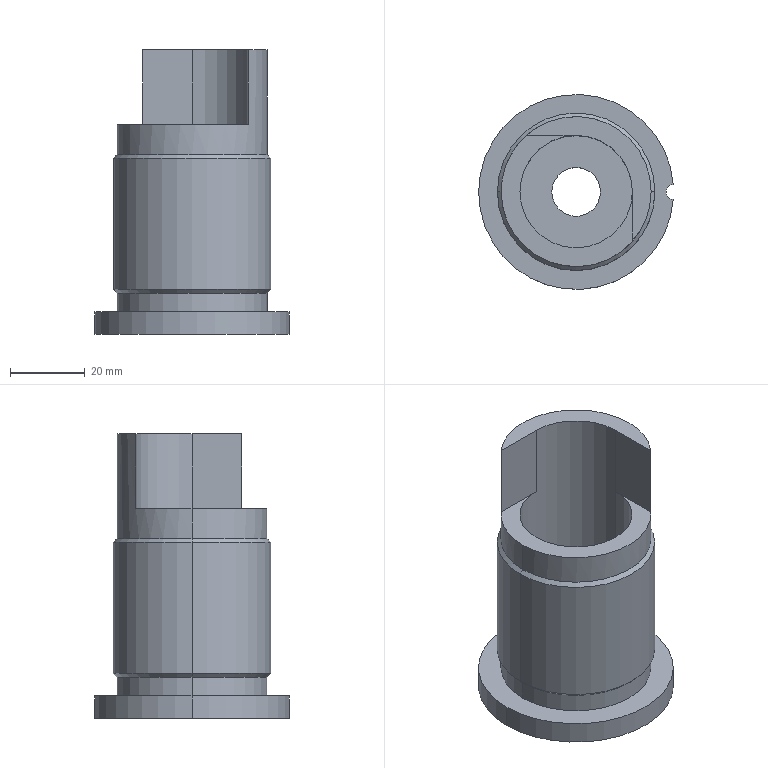Part | SolidWorks | features ICE 8, Chamfer 3, Extrusion 1 | 1 solid | 30 faces | box 51.923 x 52 x 76 mm | volume 55221 mm3 | cylinder 15 | cone 8 | plane 7 | commonest cylinder face diameters 40 x4 13 x2 30 x2 32 x2 42 x2 52 x2
STEP:
#1=CARTESIAN_POINT('',(15.,0.,21.));
#2=VERTEX_POINT('',#1);
#3=CARTESIAN_POINT('',(-15.,0.,21.));
#4=VERTEX_POINT('',#3);
#5=CARTESIAN_POINT('',(0.,0.,21.));
#6=DIRECTION('',(0.,0.,-1.));
#7=DIRECTION('',(1.,0.,0.));
#8=AXIS2_PLACEMENT_3D('',#5,#6,#7);
#9=CIRCLE('',#8,15.);
#10=EDGE_CURVE('',#2,#4,#9,.T.);
#11=ORIENTED_EDGE('',*,*,#10,.F.);
#12=CARTESIAN_POINT('',(16.,0.,20.));
#13=VERTEX_POINT('',#12);
#14=CARTESIAN_POINT('',(16.,0.,20.));
#15=DIRECTION('',(0.7071,0.,-0.7071));
#16=VECTOR('',#15,1000.);
#17=LINE('',#14,#16);
#18=EDGE_CURVE('',#2,#13,#17,.T.);
#19=ORIENTED_EDGE('',*,*,#18,.T.);
#20=CARTESIAN_POINT('',(-16.,0.,20.));
#21=VERTEX_POINT('',#20);
#22=CARTESIAN_POINT('',(0.,0.,20.));
#23=DIRECTION('',(0.,0.,1.));
#24=DIRECTION('',(1.,0.,0.));
#25=AXIS2_PLACEMENT_3D('',#22,#23,#24);
#26=CIRCLE('',#25,16.);
#27=EDGE_CURVE('',#21,#13,#26,.T.);
#28=ORIENTED_EDGE('',*,*,#27,.F.);
#29=CARTESIAN_POINT('',(-16.,0.,20.));
#30=DIRECTION('',(-0.7071,0.,-0.7071));
#31=VECTOR('',#30,1000.);
#32=LINE('',#29,#31);
#33=EDGE_CURVE('',#4,#21,#32,.T.);
#34=ORIENTED_EDGE('',*,*,#33,.F.);
#35=EDGE_LOOP('',(#11,#19,#28,#34));
#36=FACE_OUTER_BOUND('',#35,.T.);
#37=CARTESIAN_POINT('',(0.,0.,20.));
#38=DIRECTION('',(0.,0.,-1.));
#39=DIRECTION('',(-1.,0.,0.));
#40=AXIS2_PLACEMENT_3D('',#37,#38,#39);
#41=CONICAL_SURFACE('',#40,16.,0.7854);
#42=ADVANCED_FACE('',(#36),#41,.F.);
#43=CARTESIAN_POINT('',(6.5,0.,1.));
#44=VERTEX_POINT('',#43);
#45=CARTESIAN_POINT('',(-6.5,0.,1.));
#46=VERTEX_POINT('',#45);
#47=CARTESIAN_POINT('',(0.,0.,1.));
#48=DIRECTION('',(0.,0.,-1.));
#49=DIRECTION('',(1.,0.,0.));
#50=AXIS2_PLACEMENT_3D('',#47,#48,#49);
#51=CIRCLE('',#50,6.5);
#52=EDGE_CURVE('',#44,#46,#51,.T.);
#53=ORIENTED_EDGE('',*,*,#52,.F.);
#54=CARTESIAN_POINT('',(7.5,0.,0.));
#55=VERTEX_POINT('',#54);
#56=CARTESIAN_POINT('',(7.5,0.,0.));
#57=DIRECTION('',(0.7071,0.,-0.7071));
#58=VECTOR('',#57,1000.);
#59=LINE('',#56,#58);
#60=EDGE_CURVE('',#44,#55,#59,.T.);
#61=ORIENTED_EDGE('',*,*,#60,.T.);
#62=CARTESIAN_POINT('',(-7.5,0.,0.));
#63=VERTEX_POINT('',#62);
#64=CARTESIAN_POINT('',(0.,0.,0.));
#65=DIRECTION('',(0.,0.,1.));
#66=DIRECTION('',(1.,0.,0.));
#67=AXIS2_PLACEMENT_3D('',#64,#65,#66);
#68=CIRCLE('',#67,7.5);
#69=EDGE_CURVE('',#63,#55,#68,.T.);
#70=ORIENTED_EDGE('',*,*,#69,.F.);
#71=CARTESIAN_POINT('',(-7.5,0.,0.));
#72=DIRECTION('',(-0.7071,0.,-0.7071));
#73=VECTOR('',#72,1000.);
#74=LINE('',#71,#73);
#75=EDGE_CURVE('',#46,#63,#74,.T.);
#76=ORIENTED_EDGE('',*,*,#75,.F.);
#77=EDGE_LOOP('',(#53,#61,#70,#76));
#78=FACE_OUTER_BOUND('',#77,.T.);
#79=CARTESIAN_POINT('',(0.,0.,0.));
#80=DIRECTION('',(0.,0.,-1.));
#81=DIRECTION('',(-1.,0.,0.));
#82=AXIS2_PLACEMENT_3D('',#79,#80,#81);
#83=CONICAL_SURFACE('',#82,7.5,0.7854);
#84=ADVANCED_FACE('',(#78),#83,.F.);
#85=ORIENTED_EDGE('',*,*,#52,.T.);
#86=CARTESIAN_POINT('',(-6.5,0.,18.));
#87=VERTEX_POINT('',#86);
#88=CARTESIAN_POINT('',(-6.5,0.,-5.));
#89=DIRECTION('',(0.,0.,1.));
#90=VECTOR('',#89,1000.);
#91=LINE('',#88,#90);
#92=EDGE_CURVE('',#46,#87,#91,.T.);
#93=ORIENTED_EDGE('',*,*,#92,.T.);
#94=CARTESIAN_POINT('',(6.5,0.,18.));
#95=VERTEX_POINT('',#94);
#96=CARTESIAN_POINT('',(0.,0.,18.));
#97=DIRECTION('',(0.,0.,1.));
#98=DIRECTION('',(1.,0.,0.));
#99=AXIS2_PLACEMENT_3D('',#96,#97,#98);
#100=CIRCLE('',#99,6.5);
#101=EDGE_CURVE('',#87,#95,#100,.T.);
#102=ORIENTED_EDGE('',*,*,#101,.T.);
#103=CARTESIAN_POINT('',(6.5,0.,-5.));
#104=DIRECTION('',(0.,0.,1.));
#105=VECTOR('',#104,1000.);
#106=LINE('',#103,#105);
#107=EDGE_CURVE('',#44,#95,#106,.T.);
#108=ORIENTED_EDGE('',*,*,#107,.F.);
#109=EDGE_LOOP('',(#85,#93,#102,#108));
#110=FACE_OUTER_BOUND('',#109,.T.);
#111=CARTESIAN_POINT('',(0.,0.,-5.));
#112=DIRECTION('',(0.,0.,1.));
#113=DIRECTION('',(1.,0.,0.));
#114=AXIS2_PLACEMENT_3D('',#111,#112,#113);
#115=CYLINDRICAL_SURFACE('',#114,6.5);
#116=ADVANCED_FACE('',(#110),#115,.F.);
#117=ORIENTED_EDGE('',*,*,#27,.T.);
#118=CARTESIAN_POINT('',(16.,0.,18.));
#119=VERTEX_POINT('',#118);
#120=CARTESIAN_POINT('',(16.,0.,21.));
#121=DIRECTION('',(0.,0.,-1.));
#122=VECTOR('',#121,1000.);
#123=LINE('',#120,#122);
#124=EDGE_CURVE('',#13,#119,#123,.T.);
#125=ORIENTED_EDGE('',*,*,#124,.T.);
#126=CARTESIAN_POINT('',(-16.,0.,18.));
#127=VERTEX_POINT('',#126);
#128=CARTESIAN_POINT('',(0.,0.,18.));
#129=DIRECTION('',(0.,0.,1.));
#130=DIRECTION('',(1.,0.,0.));
#131=AXIS2_PLACEMENT_3D('',#128,#129,#130);
#132=CIRCLE('',#131,16.);
#133=EDGE_CURVE('',#127,#119,#132,.T.);
#134=ORIENTED_EDGE('',*,*,#133,.F.);
#135=CARTESIAN_POINT('',(-16.,0.,21.));
#136=DIRECTION('',(0.,0.,-1.));
#137=VECTOR('',#136,1000.);
#138=LINE('',#135,#137);
#139=EDGE_CURVE('',#21,#127,#138,.T.);
#140=ORIENTED_EDGE('',*,*,#139,.F.);
#141=EDGE_LOOP('',(#117,#125,#134,#140));
#142=FACE_OUTER_BOUND('',#141,.T.);
#143=CARTESIAN_POINT('',(0.,0.,21.));
#144=DIRECTION('',(0.,0.,-1.));
#145=DIRECTION('',(-1.,0.,0.));
#146=AXIS2_PLACEMENT_3D('',#143,#144,#145);
#147=CYLINDRICAL_SURFACE('',#146,16.);
#148=ADVANCED_FACE('',(#142),#147,.F.);
#149=CARTESIAN_POINT('',(-20.,0.,48.));
#150=VERTEX_POINT('',#149);
#151=CARTESIAN_POINT('',(20.,0.,48.));
#152=VERTEX_POINT('',#151);
#153=CARTESIAN_POINT('',(0.,0.,48.));
#154=DIRECTION('',(0.,0.,-1.));
#155=DIRECTION('',(1.,0.,0.));
#156=AXIS2_PLACEMENT_3D('',#153,#154,#155);
#157=CIRCLE('',#156,20.);
#158=EDGE_CURVE('',#150,#152,#157,.T.);
#159=ORIENTED_EDGE('',*,*,#158,.T.);
#160=CARTESIAN_POINT('',(21.,0.,47.));
#161=VERTEX_POINT('',#160);
#162=CARTESIAN_POINT('',(20.,0.,48.));
#163=DIRECTION('',(0.7071,0.,-0.7071));
#164=VECTOR('',#163,1000.);
#165=LINE('',#162,#164);
#166=EDGE_CURVE('',#152,#161,#165,.T.);
#167=ORIENTED_EDGE('',*,*,#166,.T.);
#168=CARTESIAN_POINT('',(-21.,0.,47.));
#169=VERTEX_POINT('',#168);
#170=CARTESIAN_POINT('',(0.,0.,47.));
#171=DIRECTION('',(0.,0.,-1.));
#172=DIRECTION('',(1.,0.,0.));
#173=AXIS2_PLACEMENT_3D('',#170,#171,#172);
#174=CIRCLE('',#173,21.);
#175=EDGE_CURVE('',#169,#161,#174,.T.);
#176=ORIENTED_EDGE('',*,*,#175,.F.);
#177=CARTESIAN_POINT('',(-20.,0.,48.));
#178=DIRECTION('',(-0.7071,0.,-0.7071));
#179=VECTOR('',#178,1000.);
#180=LINE('',#177,#179);
#181=EDGE_CURVE('',#150,#169,#180,.T.);
#182=ORIENTED_EDGE('',*,*,#181,.F.);
#183=EDGE_LOOP('',(#159,#167,#176,#182));
#184=FACE_OUTER_BOUND('',#183,.T.);
#185=CARTESIAN_POINT('',(0.,0.,48.));
#186=DIRECTION('',(0.,0.,-1.));
#187=DIRECTION('',(-1.,0.,0.));
#188=AXIS2_PLACEMENT_3D('',#185,#186,#187);
#189=CONICAL_SURFACE('',#188,20.,0.7854);
#190=ADVANCED_FACE('',(#184),#189,.T.);
#191=CARTESIAN_POINT('',(20.,0.,11.));
#192=VERTEX_POINT('',#191);
#193=CARTESIAN_POINT('',(-20.,0.,11.));
#194=VERTEX_POINT('',#193);
#195=CARTESIAN_POINT('',(0.,0.,11.));
#196=DIRECTION('',(0.,0.,1.));
#197=DIRECTION('',(1.,0.,0.));
#198=AXIS2_PLACEMENT_3D('',#195,#196,#197);
#199=CIRCLE('',#198,20.);
#200=EDGE_CURVE('',#192,#194,#199,.T.);
#201=ORIENTED_EDGE('',*,*,#200,.T.);
#202=CARTESIAN_POINT('',(-21.,0.,12.));
#203=VERTEX_POINT('',#202);
#204=CARTESIAN_POINT('',(-21.,0.,12.));
#205=DIRECTION('',(-0.7071,0.,0.7071));
#206=VECTOR('',#205,1000.);
#207=LINE('',#204,#206);
#208=EDGE_CURVE('',#194,#203,#207,.T.);
#209=ORIENTED_EDGE('',*,*,#208,.T.);
#210=CARTESIAN_POINT('',(21.,0.,12.));
#211=VERTEX_POINT('',#210);
#212=CARTESIAN_POINT('',(0.,0.,12.));
#213=DIRECTION('',(0.,0.,1.));
#214=DIRECTION('',(1.,0.,0.));
#215=AXIS2_PLACEMENT_3D('',#212,#213,#214);
#216=CIRCLE('',#215,21.);
#217=EDGE_CURVE('',#211,#203,#216,.T.);
#218=ORIENTED_EDGE('',*,*,#217,.F.);
#219=CARTESIAN_POINT('',(21.,0.,12.));
#220=DIRECTION('',(0.7071,0.,0.7071));
#221=VECTOR('',#220,1000.);
#222=LINE('',#219,#221);
#223=EDGE_CURVE('',#192,#211,#222,.T.);
#224=ORIENTED_EDGE('',*,*,#223,.F.);
#225=EDGE_LOOP('',(#201,#209,#218,#224));
#226=FACE_OUTER_BOUND('',#225,.T.);
#227=CARTESIAN_POINT('',(0.,0.,12.));
#228=DIRECTION('',(0.,0.,1.));
#229=DIRECTION('',(1.,0.,0.));
#230=AXIS2_PLACEMENT_3D('',#227,#228,#229);
#231=CONICAL_SURFACE('',#230,21.,0.7854);
#232=ADVANCED_FACE('',(#226),#231,.T.);
#233=CARTESIAN_POINT('',(20.,0.,76.));
#234=VERTEX_POINT('',#233);
#235=CARTESIAN_POINT('',(-13.229,15.,76.));
#236=VERTEX_POINT('',#235);
#237=CARTESIAN_POINT('',(0.,0.,76.));
#238=DIRECTION('',(0.,0.,1.));
#239=DIRECTION('',(1.,0.,0.));
#240=AXIS2_PLACEMENT_3D('',#237,#238,#239);
#241=CIRCLE('',#240,20.);
#242=EDGE_CURVE('',#234,#236,#241,.T.);
#243=ORIENTED_EDGE('',*,*,#242,.F.);
#244=CARTESIAN_POINT('',(20.,0.,76.));
#245=DIRECTION('',(0.,0.,-1.));
#246=VECTOR('',#245,1000.);
#247=LINE('',#244,#246);
#248=EDGE_CURVE('',#234,#152,#247,.T.);
#249=ORIENTED_EDGE('',*,*,#248,.T.);
#250=ORIENTED_EDGE('',*,*,#158,.F.);
#251=CARTESIAN_POINT('',(-20.,0.,56.));
#252=VERTEX_POINT('',#251);
#253=CARTESIAN_POINT('',(-20.,0.,76.));
#254=DIRECTION('',(0.,0.,-1.));
#255=VECTOR('',#254,1000.);
#256=LINE('',#253,#255);
#257=EDGE_CURVE('',#252,#150,#256,.T.);
#258=ORIENTED_EDGE('',*,*,#257,.F.);
#259=CARTESIAN_POINT('',(-13.229,15.,56.));
#260=VERTEX_POINT('',#259);
#261=CARTESIAN_POINT('',(0.,0.,56.));
#262=DIRECTION('',(0.,0.,1.));
#263=DIRECTION('',(1.,0.,0.));
#264=AXIS2_PLACEMENT_3D('',#261,#262,#263);
#265=CIRCLE('',#264,20.);
#266=EDGE_CURVE('',#260,#252,#265,.T.);
#267=ORIENTED_EDGE('',*,*,#266,.F.);
#268=CARTESIAN_POINT('',(-13.229,15.,76.));
#269=DIRECTION('',(0.,0.,1.));
#270=VECTOR('',#269,1000.);
#271=LINE('',#268,#270);
#272=EDGE_CURVE('',#260,#236,#271,.T.);
#273=ORIENTED_EDGE('',*,*,#272,.T.);
#274=EDGE_LOOP('',(#243,#249,#250,#258,#267,#273));
#275=FACE_OUTER_BOUND('',#274,.T.);
#276=CARTESIAN_POINT('',(0.,0.,76.));
#277=DIRECTION('',(0.,0.,-1.));
#278=DIRECTION('',(-1.,0.,0.));
#279=AXIS2_PLACEMENT_3D('',#276,#277,#278);
#280=CYLINDRICAL_SURFACE('',#279,20.);
#281=ADVANCED_FACE('',(#275),#280,.T.);
#282=ORIENTED_EDGE('',*,*,#175,.T.);
#283=CARTESIAN_POINT('',(21.,0.,48.));
#284=DIRECTION('',(0.,0.,-1.));
#285=VECTOR('',#284,1000.);
#286=LINE('',#283,#285);
#287=EDGE_CURVE('',#161,#211,#286,.T.);
#288=ORIENTED_EDGE('',*,*,#287,.T.);
#289=ORIENTED_EDGE('',*,*,#217,.T.);
#290=CARTESIAN_POINT('',(-21.,0.,48.));
#291=DIRECTION('',(0.,0.,-1.));
#292=VECTOR('',#291,1000.);
#293=LINE('',#290,#292);
#294=EDGE_CURVE('',#169,#203,#293,.T.);
#295=ORIENTED_EDGE('',*,*,#294,.F.);
#296=EDGE_LOOP('',(#282,#288,#289,#295));
#297=FACE_OUTER_BOUND('',#296,.T.);
#298=CARTESIAN_POINT('',(0.,0.,48.));
#299=DIRECTION('',(0.,0.,-1.));
#300=DIRECTION('',(-1.,0.,0.));
#301=AXIS2_PLACEMENT_3D('',#298,#299,#300);
#302=CYLINDRICAL_SURFACE('',#301,21.);
#303=ADVANCED_FACE('',(#297),#302,.T.);
#304=ORIENTED_EDGE('',*,*,#200,.F.);
#305=CARTESIAN_POINT('',(20.,0.,6.));
#306=VERTEX_POINT('',#305);
#307=CARTESIAN_POINT('',(20.,0.,11.));
#308=DIRECTION('',(0.,0.,-1.));
#309=VECTOR('',#308,1000.);
#310=LINE('',#307,#309);
#311=EDGE_CURVE('',#192,#306,#310,.T.);
#312=ORIENTED_EDGE('',*,*,#311,.T.);
#313=CARTESIAN_POINT('',(-20.,0.,6.));
#314=VERTEX_POINT('',#313);
#315=CARTESIAN_POINT('',(0.,0.,6.));
#316=DIRECTION('',(0.,0.,1.));
#317=DIRECTION('',(1.,0.,0.));
#318=AXIS2_PLACEMENT_3D('',#315,#316,#317);
#319=CIRCLE('',#318,20.);
#320=EDGE_CURVE('',#306,#314,#319,.T.);
#321=ORIENTED_EDGE('',*,*,#320,.T.);
#322=CARTESIAN_POINT('',(-20.,0.,11.));
#323=DIRECTION('',(0.,0.,-1.));
#324=VECTOR('',#323,1000.);
#325=LINE('',#322,#324);
#326=EDGE_CURVE('',#194,#314,#325,.T.);
#327=ORIENTED_EDGE('',*,*,#326,.F.);
#328=EDGE_LOOP('',(#304,#312,#321,#327));
#329=FACE_OUTER_BOUND('',#328,.T.);
#330=CARTESIAN_POINT('',(0.,0.,11.));
#331=DIRECTION('',(0.,0.,-1.));
#332=DIRECTION('',(-1.,0.,0.));
#333=AXIS2_PLACEMENT_3D('',#330,#331,#332);
#334=CYLINDRICAL_SURFACE('',#333,20.);
#335=ADVANCED_FACE('',(#329),#334,.T.);
#336=CARTESIAN_POINT('',(-26.,0.,6.));
#337=VERTEX_POINT('',#336);
#338=CARTESIAN_POINT('',(25.923,-1.999,6.));
#339=VERTEX_POINT('',#338);
#340=CARTESIAN_POINT('',(0.,0.,6.));
#341=DIRECTION('',(0.,0.,1.));
#342=DIRECTION('',(1.,0.,0.));
#343=AXIS2_PLACEMENT_3D('',#340,#341,#342);
#344=CIRCLE('',#343,26.);
#345=EDGE_CURVE('',#337,#339,#344,.T.);
#346=ORIENTED_EDGE('',*,*,#345,.F.);
#347=CARTESIAN_POINT('',(-26.,0.,0.));
#348=VERTEX_POINT('',#347);
#349=CARTESIAN_POINT('',(-26.,0.,6.));
#350=DIRECTION('',(0.,0.,-1.));
#351=VECTOR('',#350,1000.);
#352=LINE('',#349,#351);
#353=EDGE_CURVE('',#337,#348,#352,.T.);
#354=ORIENTED_EDGE('',*,*,#353,.T.);
#355=CARTESIAN_POINT('',(25.923,-1.999,0.));
#356=VERTEX_POINT('',#355);
#357=CARTESIAN_POINT('',(0.,0.,0.));
#358=DIRECTION('',(0.,0.,1.));
#359=DIRECTION('',(1.,0.,0.));
#360=AXIS2_PLACEMENT_3D('',#357,#358,#359);
#361=CIRCLE('',#360,26.);
#362=EDGE_CURVE('',#348,#356,#361,.T.);
#363=ORIENTED_EDGE('',*,*,#362,.T.);
#364=CARTESIAN_POINT('',(25.923,-1.999,-4.));
#365=DIRECTION('',(0.,0.,1.));
#366=VECTOR('',#365,1000.);
#367=LINE('',#364,#366);
#368=EDGE_CURVE('',#356,#339,#367,.T.);
#369=ORIENTED_EDGE('',*,*,#368,.T.);
#370=EDGE_LOOP('',(#346,#354,#363,#369));
#371=FACE_OUTER_BOUND('',#370,.T.);
#372=CARTESIAN_POINT('',(0.,0.,6.));
#373=DIRECTION('',(0.,0.,-1.));
#374=DIRECTION('',(-1.,0.,0.));
#375=AXIS2_PLACEMENT_3D('',#372,#373,#374);
#376=CYLINDRICAL_SURFACE('',#375,26.);
#377=ADVANCED_FACE('',(#371),#376,.T.);
#378=ORIENTED_EDGE('',*,*,#10,.T.);
#379=CARTESIAN_POINT('',(-15.,0.,56.));
#380=VERTEX_POINT('',#379);
#381=CARTESIAN_POINT('',(-15.,0.,18.));
#382=DIRECTION('',(0.,0.,1.));
#383=VECTOR('',#382,1000.);
#384=LINE('',#381,#383);
#385=EDGE_CURVE('',#4,#380,#384,.T.);
#386=ORIENTED_EDGE('',*,*,#385,.T.);
#387=CARTESIAN_POINT('',(15.,0.,56.));
#388=VERTEX_POINT('',#387);
#389=CARTESIAN_POINT('',(0.,0.,56.));
#390=DIRECTION('',(0.,0.,-1.));
#391=DIRECTION('',(1.,0.,0.));
#392=AXIS2_PLACEMENT_3D('',#389,#390,#391);
#393=CIRCLE('',#392,15.);
#394=EDGE_CURVE('',#388,#380,#393,.T.);
#395=ORIENTED_EDGE('',*,*,#394,.F.);
#396=CARTESIAN_POINT('',(15.,0.,18.));
#397=DIRECTION('',(0.,0.,1.));
#398=VECTOR('',#397,1000.);
#399=LINE('',#396,#398);
#400=EDGE_CURVE('',#2,#388,#399,.T.);
#401=ORIENTED_EDGE('',*,*,#400,.F.);
#402=EDGE_LOOP('',(#378,#386,#395,#401));
#403=FACE_OUTER_BOUND('',#402,.T.);
#404=CARTESIAN_POINT('',(0.,0.,18.));
#405=DIRECTION('',(0.,0.,1.));
#406=DIRECTION('',(1.,0.,0.));
#407=AXIS2_PLACEMENT_3D('',#404,#405,#406);
#408=CYLINDRICAL_SURFACE('',#407,15.);
#409=ADVANCED_FACE('',(#403),#408,.F.);
#410=ORIENTED_EDGE('',*,*,#385,.F.);
#411=CARTESIAN_POINT('',(0.,0.,21.));
#412=DIRECTION('',(0.,0.,-1.));
#413=DIRECTION('',(1.,0.,0.));
#414=AXIS2_PLACEMENT_3D('',#411,#412,#413);
#415=CIRCLE('',#414,15.);
#416=EDGE_CURVE('',#4,#2,#415,.T.);
#417=ORIENTED_EDGE('',*,*,#416,.T.);
#418=ORIENTED_EDGE('',*,*,#400,.T.);
#419=CARTESIAN_POINT('',(15.,0.,76.));
#420=VERTEX_POINT('',#419);
#421=CARTESIAN_POINT('',(15.,0.,56.));
#422=DIRECTION('',(0.,0.,1.));
#423=VECTOR('',#422,1000.);
#424=LINE('',#421,#423);
#425=EDGE_CURVE('',#388,#420,#424,.T.);
#426=ORIENTED_EDGE('',*,*,#425,.T.);
#427=CARTESIAN_POINT('',(0.,15.,76.));
#428=VERTEX_POINT('',#427);
#429=CARTESIAN_POINT('',(0.,0.,76.));
#430=DIRECTION('',(0.,0.,1.));
#431=DIRECTION('',(1.,0.,0.));
#432=AXIS2_PLACEMENT_3D('',#429,#430,#431);
#433=CIRCLE('',#432,15.);
#434=EDGE_CURVE('',#420,#428,#433,.T.);
#435=ORIENTED_EDGE('',*,*,#434,.T.);
#436=CARTESIAN_POINT('',(0.,15.,56.));
#437=VERTEX_POINT('',#436);
#438=CARTESIAN_POINT('',(0.,15.,56.));
#439=DIRECTION('',(0.,0.,1.));
#440=VECTOR('',#439,1000.);
#441=LINE('',#438,#440);
#442=EDGE_CURVE('',#437,#428,#441,.T.);
#443=ORIENTED_EDGE('',*,*,#442,.F.);
#444=CARTESIAN_POINT('',(0.,0.,56.));
#445=DIRECTION('',(0.,0.,-1.));
#446=DIRECTION('',(1.,0.,0.));
#447=AXIS2_PLACEMENT_3D('',#444,#445,#446);
#448=CIRCLE('',#447,15.);
#449=EDGE_CURVE('',#380,#437,#448,.T.);
#450=ORIENTED_EDGE('',*,*,#449,.F.);
#451=EDGE_LOOP('',(#410,#417,#418,#426,#435,#443,#450));
#452=FACE_OUTER_BOUND('',#451,.T.);
#453=CARTESIAN_POINT('',(0.,0.,18.));
#454=DIRECTION('',(0.,0.,1.));
#455=DIRECTION('',(1.,0.,0.));
#456=AXIS2_PLACEMENT_3D('',#453,#454,#455);
#457=CYLINDRICAL_SURFACE('',#456,15.);
#458=ADVANCED_FACE('',(#452),#457,.F.);
#459=CARTESIAN_POINT('',(25.923,1.999,6.));
#460=VERTEX_POINT('',#459);
#461=CARTESIAN_POINT('',(26.,0.,6.));
#462=DIRECTION('',(0.,0.,1.));
#463=DIRECTION('',(1.,0.,0.));
#464=AXIS2_PLACEMENT_3D('',#461,#462,#463);
#465=CIRCLE('',#464,2.);
#466=EDGE_CURVE('',#460,#339,#465,.T.);
#467=ORIENTED_EDGE('',*,*,#466,.F.);
#468=CARTESIAN_POINT('',(0.,0.,6.));
#469=DIRECTION('',(0.,0.,1.));
#470=DIRECTION('',(1.,0.,0.));
#471=AXIS2_PLACEMENT_3D('',#468,#469,#470);
#472=CIRCLE('',#471,26.);
#473=EDGE_CURVE('',#460,#337,#472,.T.);
#474=ORIENTED_EDGE('',*,*,#473,.T.);
#475=ORIENTED_EDGE('',*,*,#345,.T.);
#476=EDGE_LOOP('',(#467,#474,#475));
#477=FACE_OUTER_BOUND('',#476,.T.);
#478=CARTESIAN_POINT('',(0.,0.,6.));
#479=DIRECTION('',(0.,0.,1.));
#480=DIRECTION('',(1.,0.,0.));
#481=AXIS2_PLACEMENT_3D('',#478,#479,#480);
#482=CIRCLE('',#481,20.);
#483=EDGE_CURVE('',#314,#306,#482,.T.);
#484=ORIENTED_EDGE('',*,*,#483,.F.);
#485=ORIENTED_EDGE('',*,*,#320,.F.);
#486=EDGE_LOOP('',(#484,#485));
#487=FACE_BOUND('',#486,.T.);
#488=CARTESIAN_POINT('',(0.,0.,6.));
#489=DIRECTION('',(0.,0.,1.));
#490=DIRECTION('',(1.,0.,0.));
#491=AXIS2_PLACEMENT_3D('',#488,#489,#490);
#492=PLANE('',#491);
#493=ADVANCED_FACE('',(#477,#487),#492,.T.);
#494=ORIENTED_EDGE('',*,*,#353,.F.);
#495=ORIENTED_EDGE('',*,*,#473,.F.);
#496=CARTESIAN_POINT('',(25.923,1.999,0.));
#497=VERTEX_POINT('',#496);
#498=CARTESIAN_POINT('',(25.923,1.999,-4.));
#499=DIRECTION('',(0.,0.,-1.));
#500=VECTOR('',#499,1000.);
#501=LINE('',#498,#500);
#502=EDGE_CURVE('',#460,#497,#501,.T.);
#503=ORIENTED_EDGE('',*,*,#502,.T.);
#504=CARTESIAN_POINT('',(0.,0.,0.));
#505=DIRECTION('',(0.,0.,1.));
#506=DIRECTION('',(1.,0.,0.));
#507=AXIS2_PLACEMENT_3D('',#504,#505,#506);
#508=CIRCLE('',#507,26.);
#509=EDGE_CURVE('',#497,#348,#508,.T.);
#510=ORIENTED_EDGE('',*,*,#509,.T.);
#511=EDGE_LOOP('',(#494,#495,#503,#510));
#512=FACE_OUTER_BOUND('',#511,.T.);
#513=CARTESIAN_POINT('',(0.,0.,6.));
#514=DIRECTION('',(0.,0.,-1.));
#515=DIRECTION('',(-1.,0.,0.));
#516=AXIS2_PLACEMENT_3D('',#513,#514,#515);
#517=CYLINDRICAL_SURFACE('',#516,26.);
#518=ADVANCED_FACE('',(#512),#517,.T.);
#519=ORIENTED_EDGE('',*,*,#69,.T.);
#520=CARTESIAN_POINT('',(0.,0.,0.));
#521=DIRECTION('',(0.,0.,1.));
#522=DIRECTION('',(1.,0.,0.));
#523=AXIS2_PLACEMENT_3D('',#520,#521,#522);
#524=CIRCLE('',#523,7.5);
#525=EDGE_CURVE('',#55,#63,#524,.T.);
#526=ORIENTED_EDGE('',*,*,#525,.T.);
#527=EDGE_LOOP('',(#519,#526));
#528=FACE_BOUND('',#527,.T.);
#529=ORIENTED_EDGE('',*,*,#509,.F.);
#530=CARTESIAN_POINT('',(26.,0.,0.));
#531=DIRECTION('',(0.,0.,1.));
#532=DIRECTION('',(1.,0.,0.));
#533=AXIS2_PLACEMENT_3D('',#530,#531,#532);
#534=CIRCLE('',#533,2.);
#535=EDGE_CURVE('',#497,#356,#534,.T.);
#536=ORIENTED_EDGE('',*,*,#535,.T.);
#537=ORIENTED_EDGE('',*,*,#362,.F.);
#538=EDGE_LOOP('',(#529,#536,#537));
#539=FACE_OUTER_BOUND('',#538,.T.);
#540=CARTESIAN_POINT('',(0.,0.,0.));
#541=DIRECTION('',(0.,0.,1.));
#542=DIRECTION('',(1.,0.,0.));
#543=AXIS2_PLACEMENT_3D('',#540,#541,#542);
#544=PLANE('',#543);
#545=ADVANCED_FACE('',(#528,#539),#544,.F.);
#546=ORIENTED_EDGE('',*,*,#311,.F.);
#547=CARTESIAN_POINT('',(0.,0.,11.));
#548=DIRECTION('',(0.,0.,1.));
#549=DIRECTION('',(1.,0.,0.));
#550=AXIS2_PLACEMENT_3D('',#547,#548,#549);
#551=CIRCLE('',#550,20.);
#552=EDGE_CURVE('',#194,#192,#551,.T.);
#553=ORIENTED_EDGE('',*,*,#552,.F.);
#554=ORIENTED_EDGE('',*,*,#326,.T.);
#555=ORIENTED_EDGE('',*,*,#483,.T.);
#556=EDGE_LOOP('',(#546,#553,#554,#555));
#557=FACE_OUTER_BOUND('',#556,.T.);
#558=CARTESIAN_POINT('',(0.,0.,11.));
#559=DIRECTION('',(0.,0.,-1.));
#560=DIRECTION('',(-1.,0.,0.));
#561=AXIS2_PLACEMENT_3D('',#558,#559,#560);
#562=CYLINDRICAL_SURFACE('',#561,20.);
#563=ADVANCED_FACE('',(#557),#562,.T.);
#564=ORIENTED_EDGE('',*,*,#287,.F.);
#565=CARTESIAN_POINT('',(0.,0.,47.));
#566=DIRECTION('',(0.,0.,-1.));
#567=DIRECTION('',(1.,0.,0.));
#568=AXIS2_PLACEMENT_3D('',#565,#566,#567);
#569=CIRCLE('',#568,21.);
#570=EDGE_CURVE('',#161,#169,#569,.T.);
#571=ORIENTED_EDGE('',*,*,#570,.T.);
#572=ORIENTED_EDGE('',*,*,#294,.T.);
#573=CARTESIAN_POINT('',(0.,0.,12.));
#574=DIRECTION('',(0.,0.,1.));
#575=DIRECTION('',(1.,0.,0.));
#576=AXIS2_PLACEMENT_3D('',#573,#574,#575);
#577=CIRCLE('',#576,21.);
#578=EDGE_CURVE('',#203,#211,#577,.T.);
#579=ORIENTED_EDGE('',*,*,#578,.T.);
#580=EDGE_LOOP('',(#564,#571,#572,#579));
#581=FACE_OUTER_BOUND('',#580,.T.);
#582=CARTESIAN_POINT('',(0.,0.,48.));
#583=DIRECTION('',(0.,0.,-1.));
#584=DIRECTION('',(-1.,0.,0.));
#585=AXIS2_PLACEMENT_3D('',#582,#583,#584);
#586=CYLINDRICAL_SURFACE('',#585,21.);
#587=ADVANCED_FACE('',(#581),#586,.T.);
#588=ORIENTED_EDGE('',*,*,#248,.F.);
#589=CARTESIAN_POINT('',(15.,-13.229,76.));
#590=VERTEX_POINT('',#589);
#591=CARTESIAN_POINT('',(0.,0.,76.));
#592=DIRECTION('',(0.,0.,1.));
#593=DIRECTION('',(1.,0.,0.));
#594=AXIS2_PLACEMENT_3D('',#591,#592,#593);
#595=CIRCLE('',#594,20.);
#596=EDGE_CURVE('',#590,#234,#595,.T.);
#597=ORIENTED_EDGE('',*,*,#596,.F.);
#598=CARTESIAN_POINT('',(15.,-13.229,56.));
#599=VERTEX_POINT('',#598);
#600=CARTESIAN_POINT('',(15.,-13.229,76.));
#601=DIRECTION('',(0.,0.,-1.));
#602=VECTOR('',#601,1000.);
#603=LINE('',#600,#602);
#604=EDGE_CURVE('',#590,#599,#603,.T.);
#605=ORIENTED_EDGE('',*,*,#604,.T.);
#606=CARTESIAN_POINT('',(0.,0.,56.));
#607=DIRECTION('',(0.,0.,1.));
#608=DIRECTION('',(1.,0.,0.));
#609=AXIS2_PLACEMENT_3D('',#606,#607,#608);
#610=CIRCLE('',#609,20.);
#611=EDGE_CURVE('',#252,#599,#610,.T.);
#612=ORIENTED_EDGE('',*,*,#611,.F.);
#613=ORIENTED_EDGE('',*,*,#257,.T.);
#614=CARTESIAN_POINT('',(0.,0.,48.));
#615=DIRECTION('',(0.,0.,-1.));
#616=DIRECTION('',(1.,0.,0.));
#617=AXIS2_PLACEMENT_3D('',#614,#615,#616);
#618=CIRCLE('',#617,20.);
#619=EDGE_CURVE('',#152,#150,#618,.T.);
#620=ORIENTED_EDGE('',*,*,#619,.F.);
#621=EDGE_LOOP('',(#588,#597,#605,#612,#613,#620));
#622=FACE_OUTER_BOUND('',#621,.T.);
#623=CARTESIAN_POINT('',(0.,0.,76.));
#624=DIRECTION('',(0.,0.,-1.));
#625=DIRECTION('',(-1.,0.,0.));
#626=AXIS2_PLACEMENT_3D('',#623,#624,#625);
#627=CYLINDRICAL_SURFACE('',#626,20.);
#628=ADVANCED_FACE('',(#622),#627,.T.);
#629=CARTESIAN_POINT('',(15.,0.,76.));
#630=DIRECTION('',(0.,1.,0.));
#631=VECTOR('',#630,1000.);
#632=LINE('',#629,#631);
#633=EDGE_CURVE('',#590,#420,#632,.T.);
#634=ORIENTED_EDGE('',*,*,#633,.F.);
#635=ORIENTED_EDGE('',*,*,#596,.T.);
#636=ORIENTED_EDGE('',*,*,#242,.T.);
#637=CARTESIAN_POINT('',(0.,15.,76.));
#638=DIRECTION('',(-1.,0.,0.));
#639=VECTOR('',#638,1000.);
#640=LINE('',#637,#639);
#641=EDGE_CURVE('',#428,#236,#640,.T.);
#642=ORIENTED_EDGE('',*,*,#641,.F.);
#643=ORIENTED_EDGE('',*,*,#434,.F.);
#644=EDGE_LOOP('',(#634,#635,#636,#642,#643));
#645=FACE_OUTER_BOUND('',#644,.T.);
#646=CARTESIAN_POINT('',(0.,0.,76.));
#647=DIRECTION('',(0.,0.,1.));
#648=DIRECTION('',(1.,0.,0.));
#649=AXIS2_PLACEMENT_3D('',#646,#647,#648);
#650=PLANE('',#649);
#651=ADVANCED_FACE('',(#645),#650,.T.);
#652=ORIENTED_EDGE('',*,*,#208,.F.);
#653=ORIENTED_EDGE('',*,*,#552,.T.);
#654=ORIENTED_EDGE('',*,*,#223,.T.);
#655=ORIENTED_EDGE('',*,*,#578,.F.);
#656=EDGE_LOOP('',(#652,#653,#654,#655));
#657=FACE_OUTER_BOUND('',#656,.T.);
#658=CARTESIAN_POINT('',(0.,0.,12.));
#659=DIRECTION('',(0.,0.,1.));
#660=DIRECTION('',(1.,0.,0.));
#661=AXIS2_PLACEMENT_3D('',#658,#659,#660);
#662=CONICAL_SURFACE('',#661,21.,0.7854);
#663=ADVANCED_FACE('',(#657),#662,.T.);
#664=ORIENTED_EDGE('',*,*,#166,.F.);
#665=ORIENTED_EDGE('',*,*,#619,.T.);
#666=ORIENTED_EDGE('',*,*,#181,.T.);
#667=ORIENTED_EDGE('',*,*,#570,.F.);
#668=EDGE_LOOP('',(#664,#665,#666,#667));
#669=FACE_OUTER_BOUND('',#668,.T.);
#670=CARTESIAN_POINT('',(0.,0.,48.));
#671=DIRECTION('',(0.,0.,-1.));
#672=DIRECTION('',(-1.,0.,0.));
#673=AXIS2_PLACEMENT_3D('',#670,#671,#672);
#674=CONICAL_SURFACE('',#673,20.,0.7854);
#675=ADVANCED_FACE('',(#669),#674,.T.);
#676=ORIENTED_EDGE('',*,*,#124,.F.);
#677=CARTESIAN_POINT('',(0.,0.,20.));
#678=DIRECTION('',(0.,0.,1.));
#679=DIRECTION('',(1.,0.,0.));
#680=AXIS2_PLACEMENT_3D('',#677,#678,#679);
#681=CIRCLE('',#680,16.);
#682=EDGE_CURVE('',#13,#21,#681,.T.);
#683=ORIENTED_EDGE('',*,*,#682,.T.);
#684=ORIENTED_EDGE('',*,*,#139,.T.);
#685=CARTESIAN_POINT('',(0.,0.,18.));
#686=DIRECTION('',(0.,0.,1.));
#687=DIRECTION('',(1.,0.,0.));
#688=AXIS2_PLACEMENT_3D('',#685,#686,#687);
#689=CIRCLE('',#688,16.);
#690=EDGE_CURVE('',#119,#127,#689,.T.);
#691=ORIENTED_EDGE('',*,*,#690,.F.);
#692=EDGE_LOOP('',(#676,#683,#684,#691));
#693=FACE_OUTER_BOUND('',#692,.T.);
#694=CARTESIAN_POINT('',(0.,0.,21.));
#695=DIRECTION('',(0.,0.,-1.));
#696=DIRECTION('',(-1.,0.,0.));
#697=AXIS2_PLACEMENT_3D('',#694,#695,#696);
#698=CYLINDRICAL_SURFACE('',#697,16.);
#699=ADVANCED_FACE('',(#693),#698,.F.);
#700=CARTESIAN_POINT('',(0.,0.,18.));
#701=DIRECTION('',(0.,0.,1.));
#702=DIRECTION('',(1.,0.,0.));
#703=AXIS2_PLACEMENT_3D('',#700,#701,#702);
#704=CIRCLE('',#703,6.5);
#705=EDGE_CURVE('',#95,#87,#704,.T.);
#706=ORIENTED_EDGE('',*,*,#705,.F.);
#707=ORIENTED_EDGE('',*,*,#101,.F.);
#708=EDGE_LOOP('',(#706,#707));
#709=FACE_BOUND('',#708,.T.);
#710=ORIENTED_EDGE('',*,*,#133,.T.);
#711=ORIENTED_EDGE('',*,*,#690,.T.);
#712=EDGE_LOOP('',(#710,#711));
#713=FACE_OUTER_BOUND('',#712,.T.);
#714=CARTESIAN_POINT('',(0.,0.,18.));
#715=DIRECTION('',(0.,0.,1.));
#716=DIRECTION('',(1.,0.,0.));
#717=AXIS2_PLACEMENT_3D('',#714,#715,#716);
#718=PLANE('',#717);
#719=ADVANCED_FACE('',(#709,#713),#718,.T.);
#720=ORIENTED_EDGE('',*,*,#92,.F.);
#721=CARTESIAN_POINT('',(0.,0.,1.));
#722=DIRECTION('',(0.,0.,-1.));
#723=DIRECTION('',(1.,0.,0.));
#724=AXIS2_PLACEMENT_3D('',#721,#722,#723);
#725=CIRCLE('',#724,6.5);
#726=EDGE_CURVE('',#46,#44,#725,.T.);
#727=ORIENTED_EDGE('',*,*,#726,.T.);
#728=ORIENTED_EDGE('',*,*,#107,.T.);
#729=ORIENTED_EDGE('',*,*,#705,.T.);
#730=EDGE_LOOP('',(#720,#727,#728,#729));
#731=FACE_OUTER_BOUND('',#730,.T.);
#732=CARTESIAN_POINT('',(0.,0.,-5.));
#733=DIRECTION('',(0.,0.,1.));
#734=DIRECTION('',(1.,0.,0.));
#735=AXIS2_PLACEMENT_3D('',#732,#733,#734);
#736=CYLINDRICAL_SURFACE('',#735,6.5);
#737=ADVANCED_FACE('',(#731),#736,.F.);
#738=ORIENTED_EDGE('',*,*,#633,.T.);
#739=ORIENTED_EDGE('',*,*,#425,.F.);
#740=CARTESIAN_POINT('',(15.,0.,56.));
#741=DIRECTION('',(0.,1.,0.));
#742=VECTOR('',#741,1000.);
#743=LINE('',#740,#742);
#744=EDGE_CURVE('',#599,#388,#743,.T.);
#745=ORIENTED_EDGE('',*,*,#744,.F.);
#746=ORIENTED_EDGE('',*,*,#604,.F.);
#747=EDGE_LOOP('',(#738,#739,#745,#746));
#748=FACE_OUTER_BOUND('',#747,.T.);
#749=CARTESIAN_POINT('',(15.,0.,56.));
#750=DIRECTION('',(1.,0.,0.));
#751=DIRECTION('',(0.,1.,0.));
#752=AXIS2_PLACEMENT_3D('',#749,#750,#751);
#753=PLANE('',#752);
#754=ADVANCED_FACE('',(#748),#753,.F.);
#755=CARTESIAN_POINT('',(0.,15.,56.));
#756=DIRECTION('',(-1.,0.,0.));
#757=VECTOR('',#756,1000.);
#758=LINE('',#755,#757);
#759=EDGE_CURVE('',#437,#260,#758,.T.);
#760=ORIENTED_EDGE('',*,*,#759,.F.);
#761=ORIENTED_EDGE('',*,*,#442,.T.);
#762=ORIENTED_EDGE('',*,*,#641,.T.);
#763=ORIENTED_EDGE('',*,*,#272,.F.);
#764=EDGE_LOOP('',(#760,#761,#762,#763));
#765=FACE_OUTER_BOUND('',#764,.T.);
#766=CARTESIAN_POINT('',(0.,15.,56.));
#767=DIRECTION('',(0.,1.,0.));
#768=DIRECTION('',(-1.,0.,0.));
#769=AXIS2_PLACEMENT_3D('',#766,#767,#768);
#770=PLANE('',#769);
#771=ADVANCED_FACE('',(#765),#770,.F.);
#772=ORIENTED_EDGE('',*,*,#266,.T.);
#773=ORIENTED_EDGE('',*,*,#611,.T.);
#774=ORIENTED_EDGE('',*,*,#744,.T.);
#775=ORIENTED_EDGE('',*,*,#394,.T.);
#776=ORIENTED_EDGE('',*,*,#449,.T.);
#777=ORIENTED_EDGE('',*,*,#759,.T.);
#778=EDGE_LOOP('',(#772,#773,#774,#775,#776,#777));
#779=FACE_OUTER_BOUND('',#778,.T.);
#780=CARTESIAN_POINT('',(0.,0.,56.));
#781=DIRECTION('',(0.,0.,1.));
#782=DIRECTION('',(1.,0.,0.));
#783=AXIS2_PLACEMENT_3D('',#780,#781,#782);
#784=PLANE('',#783);
#785=ADVANCED_FACE('',(#779),#784,.T.);
#786=ORIENTED_EDGE('',*,*,#535,.F.);
#787=ORIENTED_EDGE('',*,*,#502,.F.);
#788=ORIENTED_EDGE('',*,*,#466,.T.);
#789=ORIENTED_EDGE('',*,*,#368,.F.);
#790=EDGE_LOOP('',(#786,#787,#788,#789));
#791=FACE_OUTER_BOUND('',#790,.T.);
#792=CARTESIAN_POINT('',(26.,0.,-14.));
#793=DIRECTION('',(0.,0.,1.));
#794=DIRECTION('',(1.,0.,0.));
#795=AXIS2_PLACEMENT_3D('',#792,#793,#794);
#796=CYLINDRICAL_SURFACE('',#795,2.);
#797=ADVANCED_FACE('',(#791),#796,.F.);
#798=ORIENTED_EDGE('',*,*,#60,.F.);
#799=ORIENTED_EDGE('',*,*,#726,.F.);
#800=ORIENTED_EDGE('',*,*,#75,.T.);
#801=ORIENTED_EDGE('',*,*,#525,.F.);
#802=EDGE_LOOP('',(#798,#799,#800,#801));
#803=FACE_OUTER_BOUND('',#802,.T.);
#804=CARTESIAN_POINT('',(0.,0.,0.));
#805=DIRECTION('',(0.,0.,-1.));
#806=DIRECTION('',(-1.,0.,0.));
#807=AXIS2_PLACEMENT_3D('',#804,#805,#806);
#808=CONICAL_SURFACE('',#807,7.5,0.7854);
#809=ADVANCED_FACE('',(#803),#808,.F.);
#810=ORIENTED_EDGE('',*,*,#18,.F.);
#811=ORIENTED_EDGE('',*,*,#416,.F.);
#812=ORIENTED_EDGE('',*,*,#33,.T.);
#813=ORIENTED_EDGE('',*,*,#682,.F.);
#814=EDGE_LOOP('',(#810,#811,#812,#813));
#815=FACE_OUTER_BOUND('',#814,.T.);
#816=CARTESIAN_POINT('',(0.,0.,20.));
#817=DIRECTION('',(0.,0.,-1.));
#818=DIRECTION('',(-1.,0.,0.));
#819=AXIS2_PLACEMENT_3D('',#816,#817,#818);
#820=CONICAL_SURFACE('',#819,16.,0.7854);
#821=ADVANCED_FACE('',(#815),#820,.F.);
#822=CLOSED_SHELL('',(#42,#84,#116,#148,#190,#232,#281,#303,#335,#377,#409,#458,#493,#518,#545,#563,#587,#628,#651,#663,#675,#699,#719,#737,#754,#771,#785,#797,#809,#821));
#823=MANIFOLD_SOLID_BREP('',#822);
#824=CARTESIAN_POINT('',(0.,0.,0.));
#825=DIRECTION('',(0.,0.,1.));
#826=DIRECTION('',(1.,0.,0.));
#827=AXIS2_PLACEMENT_3D('',#824,#825,#826);
#828=(LENGTH_UNIT()NAMED_UNIT(*)SI_UNIT(.MILLI.,.METRE.));
#829=UNCERTAINTY_MEASURE_WITH_UNIT(LENGTH_MEASURE(0.00001),#828,'','');
#830=(NAMED_UNIT(*)PLANE_ANGLE_UNIT()SI_UNIT($,.RADIAN.));
#831=(NAMED_UNIT(*)SI_UNIT($,.STERADIAN.)SOLID_ANGLE_UNIT());
#832=(GEOMETRIC_REPRESENTATION_CONTEXT(3)GLOBAL_UNCERTAINTY_ASSIGNED_CONTEXT((#829))GLOBAL_UNIT_ASSIGNED_CONTEXT((#828,#830,#831))REPRESENTATION_CONTEXT('',''));
#833=ADVANCED_BREP_SHAPE_REPRESENTATION('',(#823,#827),#832);